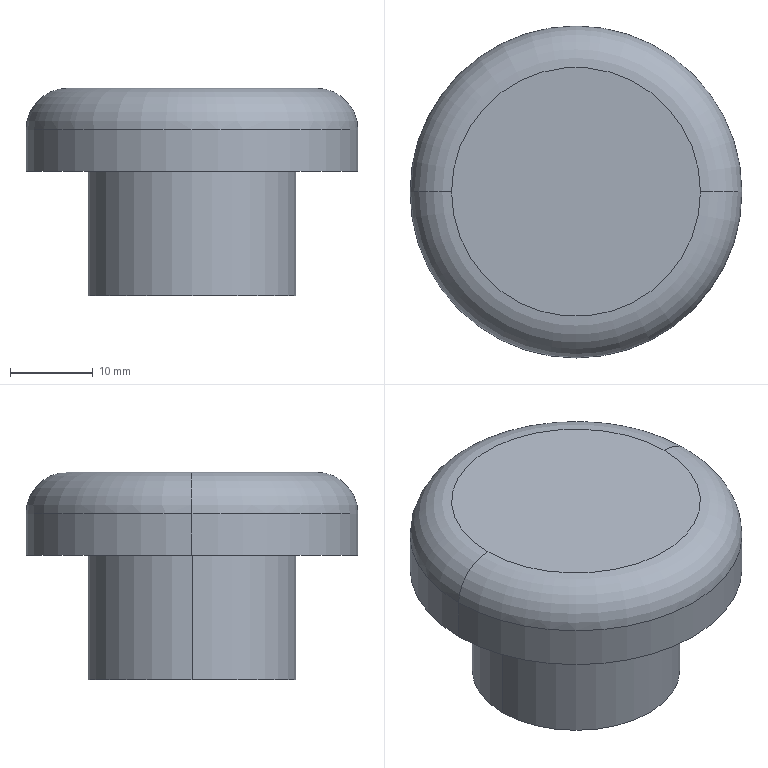Part | STEP file | 7-4-Emergency Stop Button1-619-724_Default | 1 solid | 9 faces | box 40 x 40 x 25 mm | volume 19293 mm3 | cylinder 4 | plane 3 | torus 2 | commonest cylinder face diameters 25 x2 40 x2
STEP:
#1=CARTESIAN_POINT('',(0.,0.,0.));
#2=DIRECTION('',(0.,0.,1.));
#3=DIRECTION('',(1.,0.,0.));
#4=AXIS2_PLACEMENT_3D('',#1,#2,#3);
#5=CARTESIAN_POINT('',(-20.,0.,-5.));
#6=VERTEX_POINT('',#5);
#7=CARTESIAN_POINT('',(20.,0.,-5.));
#8=VERTEX_POINT('',#7);
#9=CARTESIAN_POINT('',(0.,0.,-5.));
#10=DIRECTION('',(0.,0.,-1.));
#11=DIRECTION('',(1.,0.,0.));
#12=AXIS2_PLACEMENT_3D('',#9,#10,#11);
#13=CIRCLE('',#12,20.);
#14=CARTESIAN_POINT('',(0.,0.,-5.));
#15=DIRECTION('',(0.,0.,1.));
#16=DIRECTION('',(1.,0.,0.));
#17=AXIS2_PLACEMENT_3D('',#14,#15,#16);
#18=TOROIDAL_SURFACE('',#17,15.,5.);
#19=CARTESIAN_POINT('',(6.283,0.));
#20=DIRECTION('',(-1.,0.));
#21=VECTOR('',#20,1.);
#22=LINE('',#19,#21);
#23=(GEOMETRIC_REPRESENTATION_CONTEXT(2)PARAMETRIC_REPRESENTATION_CONTEXT()REPRESENTATION_CONTEXT('',''));
#24=DEFINITIONAL_REPRESENTATION('',(#22),#23);
#25=PCURVE('',#18,#24);
#26=CARTESIAN_POINT('',(0.,0.,-25.));
#27=DIRECTION('',(0.,0.,1.));
#28=DIRECTION('',(1.,0.,0.));
#29=AXIS2_PLACEMENT_3D('',#26,#27,#28);
#30=CYLINDRICAL_SURFACE('',#29,20.);
#31=CARTESIAN_POINT('',(6.283,20.));
#32=DIRECTION('',(-1.,0.));
#33=VECTOR('',#32,1.);
#34=LINE('',#31,#33);
#35=(GEOMETRIC_REPRESENTATION_CONTEXT(2)PARAMETRIC_REPRESENTATION_CONTEXT()REPRESENTATION_CONTEXT('',''));
#36=DEFINITIONAL_REPRESENTATION('',(#34),#35);
#37=PCURVE('',#30,#36);
#38=SURFACE_CURVE('',#13,(#25,#37),.PCURVE_S1.);
#39=EDGE_CURVE('',#6,#8,#38,.T.);
#40=ORIENTED_EDGE('',*,*,#39,.F.);
#41=CARTESIAN_POINT('',(-15.,0.,0.));
#42=VERTEX_POINT('',#41);
#43=CARTESIAN_POINT('',(-15.,0.,-5.));
#44=DIRECTION('',(0.,1.,0.));
#45=DIRECTION('',(-1.,0.,0.));
#46=AXIS2_PLACEMENT_3D('',#43,#44,#45);
#47=CIRCLE('',#46,5.);
#48=CARTESIAN_POINT('',(3.142,0.));
#49=DIRECTION('',(0.,1.));
#50=VECTOR('',#49,1.);
#51=LINE('',#48,#50);
#52=(GEOMETRIC_REPRESENTATION_CONTEXT(2)PARAMETRIC_REPRESENTATION_CONTEXT()REPRESENTATION_CONTEXT('',''));
#53=DEFINITIONAL_REPRESENTATION('',(#51),#52);
#54=PCURVE('',#18,#53);
#55=CARTESIAN_POINT('',(0.,0.,-5.));
#56=DIRECTION('',(0.,0.,1.));
#57=DIRECTION('',(1.,0.,0.));
#58=AXIS2_PLACEMENT_3D('',#55,#56,#57);
#59=TOROIDAL_SURFACE('',#58,15.,5.);
#60=CARTESIAN_POINT('',(3.142,0.));
#61=DIRECTION('',(0.,1.));
#62=VECTOR('',#61,1.);
#63=LINE('',#60,#62);
#64=(GEOMETRIC_REPRESENTATION_CONTEXT(2)PARAMETRIC_REPRESENTATION_CONTEXT()REPRESENTATION_CONTEXT('',''));
#65=DEFINITIONAL_REPRESENTATION('',(#63),#64);
#66=PCURVE('',#59,#65);
#67=SURFACE_CURVE('',#47,(#54,#66),.PCURVE_S1.);
#68=EDGE_CURVE('',#6,#42,#67,.T.);
#69=ORIENTED_EDGE('',*,*,#68,.T.);
#70=CARTESIAN_POINT('',(15.,0.,0.));
#71=VERTEX_POINT('',#70);
#72=CARTESIAN_POINT('',(0.,0.,0.));
#73=DIRECTION('',(0.,0.,1.));
#74=DIRECTION('',(1.,0.,0.));
#75=AXIS2_PLACEMENT_3D('',#72,#73,#74);
#76=CIRCLE('',#75,15.);
#77=CARTESIAN_POINT('',(0.,1.571));
#78=DIRECTION('',(1.,0.));
#79=VECTOR('',#78,1.);
#80=LINE('',#77,#79);
#81=(GEOMETRIC_REPRESENTATION_CONTEXT(2)PARAMETRIC_REPRESENTATION_CONTEXT()REPRESENTATION_CONTEXT('',''));
#82=DEFINITIONAL_REPRESENTATION('',(#80),#81);
#83=PCURVE('',#18,#82);
#84=CARTESIAN_POINT('',(0.,0.,0.));
#85=DIRECTION('',(0.,0.,1.));
#86=DIRECTION('',(1.,0.,0.));
#87=AXIS2_PLACEMENT_3D('',#84,#85,#86);
#88=PLANE('',#87);
#89=CARTESIAN_POINT('',(0.,0.));
#90=DIRECTION('',(1.,0.));
#91=AXIS2_PLACEMENT_2D('',#89,#90);
#92=CIRCLE('',#91,15.);
#93=(GEOMETRIC_REPRESENTATION_CONTEXT(2)PARAMETRIC_REPRESENTATION_CONTEXT()REPRESENTATION_CONTEXT('',''));
#94=DEFINITIONAL_REPRESENTATION('',(#92),#93);
#95=PCURVE('',#88,#94);
#96=SURFACE_CURVE('',#76,(#83,#95),.PCURVE_S1.);
#97=EDGE_CURVE('',#71,#42,#96,.T.);
#98=ORIENTED_EDGE('',*,*,#97,.F.);
#99=CARTESIAN_POINT('',(15.,0.,-5.));
#100=DIRECTION('',(0.,-1.,0.));
#101=DIRECTION('',(0.,0.,-1.));
#102=AXIS2_PLACEMENT_3D('',#99,#100,#101);
#103=CIRCLE('',#102,5.);
#104=CARTESIAN_POINT('',(0.,-1.571));
#105=DIRECTION('',(0.,1.));
#106=VECTOR('',#105,1.);
#107=LINE('',#104,#106);
#108=(GEOMETRIC_REPRESENTATION_CONTEXT(2)PARAMETRIC_REPRESENTATION_CONTEXT()REPRESENTATION_CONTEXT('',''));
#109=DEFINITIONAL_REPRESENTATION('',(#107),#108);
#110=PCURVE('',#18,#109);
#111=CARTESIAN_POINT('',(6.283,-1.571));
#112=DIRECTION('',(0.,1.));
#113=VECTOR('',#112,1.);
#114=LINE('',#111,#113);
#115=(GEOMETRIC_REPRESENTATION_CONTEXT(2)PARAMETRIC_REPRESENTATION_CONTEXT()REPRESENTATION_CONTEXT('',''));
#116=DEFINITIONAL_REPRESENTATION('',(#114),#115);
#117=PCURVE('',#59,#116);
#118=SURFACE_CURVE('',#103,(#110,#117),.PCURVE_S1.);
#119=EDGE_CURVE('',#8,#71,#118,.T.);
#120=ORIENTED_EDGE('',*,*,#119,.F.);
#121=EDGE_LOOP('',(#40,#69,#98,#120));
#122=FACE_BOUND('',#121,.T.);
#123=ADVANCED_FACE('',(#122),#18,.T.);
#124=CARTESIAN_POINT('',(-12.5,0.,-10.));
#125=VERTEX_POINT('',#124);
#126=CARTESIAN_POINT('',(12.5,0.,-10.));
#127=VERTEX_POINT('',#126);
#128=CARTESIAN_POINT('',(0.,0.,-10.));
#129=DIRECTION('',(0.,0.,-1.));
#130=DIRECTION('',(-1.,0.,0.));
#131=AXIS2_PLACEMENT_3D('',#128,#129,#130);
#132=CIRCLE('',#131,12.5);
#133=CARTESIAN_POINT('',(0.,0.,-10.));
#134=DIRECTION('',(0.,0.,-1.));
#135=DIRECTION('',(-1.,0.,0.));
#136=AXIS2_PLACEMENT_3D('',#133,#134,#135);
#137=CYLINDRICAL_SURFACE('',#136,12.5);
#138=CARTESIAN_POINT('',(0.,0.));
#139=DIRECTION('',(1.,0.));
#140=VECTOR('',#139,1.);
#141=LINE('',#138,#140);
#142=(GEOMETRIC_REPRESENTATION_CONTEXT(2)PARAMETRIC_REPRESENTATION_CONTEXT()REPRESENTATION_CONTEXT('',''));
#143=DEFINITIONAL_REPRESENTATION('',(#141),#142);
#144=PCURVE('',#137,#143);
#145=CARTESIAN_POINT('',(0.,0.,-10.));
#146=DIRECTION('',(0.,0.,-1.));
#147=DIRECTION('',(-1.,0.,0.));
#148=AXIS2_PLACEMENT_3D('',#145,#146,#147);
#149=PLANE('',#148);
#150=CARTESIAN_POINT('',(0.,0.));
#151=DIRECTION('',(1.,0.));
#152=AXIS2_PLACEMENT_2D('',#150,#151);
#153=CIRCLE('',#152,12.5);
#154=(GEOMETRIC_REPRESENTATION_CONTEXT(2)PARAMETRIC_REPRESENTATION_CONTEXT()REPRESENTATION_CONTEXT('',''));
#155=DEFINITIONAL_REPRESENTATION('',(#153),#154);
#156=PCURVE('',#149,#155);
#157=SURFACE_CURVE('',#132,(#144,#156),.PCURVE_S1.);
#158=EDGE_CURVE('',#125,#127,#157,.T.);
#159=ORIENTED_EDGE('',*,*,#158,.T.);
#160=CARTESIAN_POINT('',(12.5,0.,-25.));
#161=VERTEX_POINT('',#160);
#162=CARTESIAN_POINT('',(12.5,0.,-10.));
#163=DIRECTION('',(0.,0.,-1.));
#164=VECTOR('',#163,1.);
#165=LINE('',#162,#164);
#166=CARTESIAN_POINT('',(3.142,0.));
#167=DIRECTION('',(0.,1.));
#168=VECTOR('',#167,1.);
#169=LINE('',#166,#168);
#170=(GEOMETRIC_REPRESENTATION_CONTEXT(2)PARAMETRIC_REPRESENTATION_CONTEXT()REPRESENTATION_CONTEXT('',''));
#171=DEFINITIONAL_REPRESENTATION('',(#169),#170);
#172=PCURVE('',#137,#171);
#173=CARTESIAN_POINT('',(0.,0.,-10.));
#174=DIRECTION('',(0.,0.,-1.));
#175=DIRECTION('',(-1.,0.,0.));
#176=AXIS2_PLACEMENT_3D('',#173,#174,#175);
#177=CYLINDRICAL_SURFACE('',#176,12.5);
#178=CARTESIAN_POINT('',(3.142,0.));
#179=DIRECTION('',(0.,1.));
#180=VECTOR('',#179,1.);
#181=LINE('',#178,#180);
#182=(GEOMETRIC_REPRESENTATION_CONTEXT(2)PARAMETRIC_REPRESENTATION_CONTEXT()REPRESENTATION_CONTEXT('',''));
#183=DEFINITIONAL_REPRESENTATION('',(#181),#182);
#184=PCURVE('',#177,#183);
#185=SURFACE_CURVE('',#165,(#172,#184),.PCURVE_S1.);
#186=EDGE_CURVE('',#127,#161,#185,.T.);
#187=ORIENTED_EDGE('',*,*,#186,.T.);
#188=CARTESIAN_POINT('',(-12.5,0.,-25.));
#189=VERTEX_POINT('',#188);
#190=CARTESIAN_POINT('',(0.,0.,-25.));
#191=DIRECTION('',(0.,0.,-1.));
#192=DIRECTION('',(-1.,0.,0.));
#193=AXIS2_PLACEMENT_3D('',#190,#191,#192);
#194=CIRCLE('',#193,12.5);
#195=CARTESIAN_POINT('',(0.,15.));
#196=DIRECTION('',(1.,0.));
#197=VECTOR('',#196,1.);
#198=LINE('',#195,#197);
#199=(GEOMETRIC_REPRESENTATION_CONTEXT(2)PARAMETRIC_REPRESENTATION_CONTEXT()REPRESENTATION_CONTEXT('',''));
#200=DEFINITIONAL_REPRESENTATION('',(#198),#199);
#201=PCURVE('',#137,#200);
#202=CARTESIAN_POINT('',(0.,0.,-25.));
#203=DIRECTION('',(0.,0.,1.));
#204=DIRECTION('',(1.,0.,0.));
#205=AXIS2_PLACEMENT_3D('',#202,#203,#204);
#206=PLANE('',#205);
#207=CARTESIAN_POINT('',(-12.5,0.));
#208=CARTESIAN_POINT('',(-12.5,21.651));
#209=CARTESIAN_POINT('',(6.25,10.825));
#210=CARTESIAN_POINT('',(25.,0.));
#211=CARTESIAN_POINT('',(6.25,-10.825));
#212=CARTESIAN_POINT('',(-12.5,-21.651));
#213=CARTESIAN_POINT('',(-12.5,0.));
#214=(BOUNDED_CURVE()B_SPLINE_CURVE(2,(#207,#208,#209,#210,#211,#212,#213),.UNSPECIFIED.,.T.,.F.)B_SPLINE_CURVE_WITH_KNOTS((1,2,2,2,2,1),(-2.094,0.,2.094,4.189,6.283,8.378),.UNSPECIFIED.)CURVE()GEOMETRIC_REPRESENTATION_ITEM()RATIONAL_B_SPLINE_CURVE((1.,0.5,1.,0.5,1.,0.5,1.))REPRESENTATION_ITEM(''));
#215=(GEOMETRIC_REPRESENTATION_CONTEXT(2)PARAMETRIC_REPRESENTATION_CONTEXT()REPRESENTATION_CONTEXT('',''));
#216=DEFINITIONAL_REPRESENTATION('',(#214),#215);
#217=PCURVE('',#206,#216);
#218=SURFACE_CURVE('',#194,(#201,#217),.PCURVE_S1.);
#219=EDGE_CURVE('',#189,#161,#218,.T.);
#220=ORIENTED_EDGE('',*,*,#219,.F.);
#221=CARTESIAN_POINT('',(-12.5,0.,-10.));
#222=DIRECTION('',(0.,0.,-1.));
#223=VECTOR('',#222,1.);
#224=LINE('',#221,#223);
#225=CARTESIAN_POINT('',(0.,0.));
#226=DIRECTION('',(0.,1.));
#227=VECTOR('',#226,1.);
#228=LINE('',#225,#227);
#229=(GEOMETRIC_REPRESENTATION_CONTEXT(2)PARAMETRIC_REPRESENTATION_CONTEXT()REPRESENTATION_CONTEXT('',''));
#230=DEFINITIONAL_REPRESENTATION('',(#228),#229);
#231=PCURVE('',#137,#230);
#232=CARTESIAN_POINT('',(6.283,0.));
#233=DIRECTION('',(0.,1.));
#234=VECTOR('',#233,1.);
#235=LINE('',#232,#234);
#236=(GEOMETRIC_REPRESENTATION_CONTEXT(2)PARAMETRIC_REPRESENTATION_CONTEXT()REPRESENTATION_CONTEXT('',''));
#237=DEFINITIONAL_REPRESENTATION('',(#235),#236);
#238=PCURVE('',#177,#237);
#239=SURFACE_CURVE('',#224,(#231,#238),.PCURVE_S1.);
#240=EDGE_CURVE('',#125,#189,#239,.T.);
#241=ORIENTED_EDGE('',*,*,#240,.F.);
#242=EDGE_LOOP('',(#159,#187,#220,#241));
#243=FACE_BOUND('',#242,.T.);
#244=ADVANCED_FACE('',(#243),#137,.T.);
#245=CARTESIAN_POINT('',(20.,0.,-10.));
#246=VERTEX_POINT('',#245);
#247=CARTESIAN_POINT('',(-20.,0.,-10.));
#248=VERTEX_POINT('',#247);
#249=CARTESIAN_POINT('',(0.,0.,-10.));
#250=DIRECTION('',(0.,0.,1.));
#251=DIRECTION('',(-1.,0.,0.));
#252=AXIS2_PLACEMENT_3D('',#249,#250,#251);
#253=CIRCLE('',#252,20.);
#254=CARTESIAN_POINT('',(-3.142,15.));
#255=DIRECTION('',(1.,0.));
#256=VECTOR('',#255,1.);
#257=LINE('',#254,#256);
#258=(GEOMETRIC_REPRESENTATION_CONTEXT(2)PARAMETRIC_REPRESENTATION_CONTEXT()REPRESENTATION_CONTEXT('',''));
#259=DEFINITIONAL_REPRESENTATION('',(#257),#258);
#260=PCURVE('',#30,#259);
#261=CARTESIAN_POINT('',(20.,0.));
#262=CARTESIAN_POINT('',(20.,-34.641));
#263=CARTESIAN_POINT('',(-10.,-17.321));
#264=CARTESIAN_POINT('',(-40.,0.));
#265=CARTESIAN_POINT('',(-10.,17.321));
#266=CARTESIAN_POINT('',(20.,34.641));
#267=CARTESIAN_POINT('',(20.,0.));
#268=(BOUNDED_CURVE()B_SPLINE_CURVE(2,(#261,#262,#263,#264,#265,#266,#267),.UNSPECIFIED.,.T.,.F.)B_SPLINE_CURVE_WITH_KNOTS((1,2,2,2,2,1),(-2.094,0.,2.094,4.189,6.283,8.378),.UNSPECIFIED.)CURVE()GEOMETRIC_REPRESENTATION_ITEM()RATIONAL_B_SPLINE_CURVE((1.,0.5,1.,0.5,1.,0.5,1.))REPRESENTATION_ITEM(''));
#269=(GEOMETRIC_REPRESENTATION_CONTEXT(2)PARAMETRIC_REPRESENTATION_CONTEXT()REPRESENTATION_CONTEXT('',''));
#270=DEFINITIONAL_REPRESENTATION('',(#268),#269);
#271=PCURVE('',#149,#270);
#272=SURFACE_CURVE('',#253,(#260,#271),.PCURVE_S1.);
#273=EDGE_CURVE('',#246,#248,#272,.T.);
#274=ORIENTED_EDGE('',*,*,#273,.T.);
#275=CARTESIAN_POINT('',(-20.,0.,-25.));
#276=DIRECTION('',(0.,0.,1.));
#277=VECTOR('',#276,1.);
#278=LINE('',#275,#277);
#279=CARTESIAN_POINT('',(3.142,0.));
#280=DIRECTION('',(0.,1.));
#281=VECTOR('',#280,1.);
#282=LINE('',#279,#281);
#283=(GEOMETRIC_REPRESENTATION_CONTEXT(2)PARAMETRIC_REPRESENTATION_CONTEXT()REPRESENTATION_CONTEXT('',''));
#284=DEFINITIONAL_REPRESENTATION('',(#282),#283);
#285=PCURVE('',#30,#284);
#286=CARTESIAN_POINT('',(0.,0.,-25.));
#287=DIRECTION('',(0.,0.,1.));
#288=DIRECTION('',(1.,0.,0.));
#289=AXIS2_PLACEMENT_3D('',#286,#287,#288);
#290=CYLINDRICAL_SURFACE('',#289,20.);
#291=CARTESIAN_POINT('',(3.142,0.));
#292=DIRECTION('',(0.,1.));
#293=VECTOR('',#292,1.);
#294=LINE('',#291,#293);
#295=(GEOMETRIC_REPRESENTATION_CONTEXT(2)PARAMETRIC_REPRESENTATION_CONTEXT()REPRESENTATION_CONTEXT('',''));
#296=DEFINITIONAL_REPRESENTATION('',(#294),#295);
#297=PCURVE('',#290,#296);
#298=SURFACE_CURVE('',#278,(#285,#297),.PCURVE_S1.);
#299=EDGE_CURVE('',#248,#6,#298,.T.);
#300=ORIENTED_EDGE('',*,*,#299,.T.);
#301=ORIENTED_EDGE('',*,*,#39,.T.);
#302=CARTESIAN_POINT('',(20.,0.,-25.));
#303=DIRECTION('',(0.,0.,1.));
#304=VECTOR('',#303,1.);
#305=LINE('',#302,#304);
#306=CARTESIAN_POINT('',(0.,0.));
#307=DIRECTION('',(0.,1.));
#308=VECTOR('',#307,1.);
#309=LINE('',#306,#308);
#310=(GEOMETRIC_REPRESENTATION_CONTEXT(2)PARAMETRIC_REPRESENTATION_CONTEXT()REPRESENTATION_CONTEXT('',''));
#311=DEFINITIONAL_REPRESENTATION('',(#309),#310);
#312=PCURVE('',#30,#311);
#313=CARTESIAN_POINT('',(6.283,0.));
#314=DIRECTION('',(0.,1.));
#315=VECTOR('',#314,1.);
#316=LINE('',#313,#315);
#317=(GEOMETRIC_REPRESENTATION_CONTEXT(2)PARAMETRIC_REPRESENTATION_CONTEXT()REPRESENTATION_CONTEXT('',''));
#318=DEFINITIONAL_REPRESENTATION('',(#316),#317);
#319=PCURVE('',#290,#318);
#320=SURFACE_CURVE('',#305,(#312,#319),.PCURVE_S1.);
#321=EDGE_CURVE('',#246,#8,#320,.T.);
#322=ORIENTED_EDGE('',*,*,#321,.F.);
#323=EDGE_LOOP('',(#274,#300,#301,#322));
#324=FACE_BOUND('',#323,.T.);
#325=ADVANCED_FACE('',(#324),#30,.T.);
#326=ORIENTED_EDGE('',*,*,#299,.F.);
#327=CARTESIAN_POINT('',(0.,0.,-10.));
#328=DIRECTION('',(0.,0.,1.));
#329=DIRECTION('',(-1.,0.,0.));
#330=AXIS2_PLACEMENT_3D('',#327,#328,#329);
#331=CIRCLE('',#330,20.);
#332=CARTESIAN_POINT('',(3.142,15.));
#333=DIRECTION('',(1.,0.));
#334=VECTOR('',#333,1.);
#335=LINE('',#332,#334);
#336=(GEOMETRIC_REPRESENTATION_CONTEXT(2)PARAMETRIC_REPRESENTATION_CONTEXT()REPRESENTATION_CONTEXT('',''));
#337=DEFINITIONAL_REPRESENTATION('',(#335),#336);
#338=PCURVE('',#290,#337);
#339=CARTESIAN_POINT('',(20.,0.));
#340=CARTESIAN_POINT('',(20.,-34.641));
#341=CARTESIAN_POINT('',(-10.,-17.321));
#342=CARTESIAN_POINT('',(-40.,0.));
#343=CARTESIAN_POINT('',(-10.,17.321));
#344=CARTESIAN_POINT('',(20.,34.641));
#345=CARTESIAN_POINT('',(20.,0.));
#346=(BOUNDED_CURVE()B_SPLINE_CURVE(2,(#339,#340,#341,#342,#343,#344,#345),.UNSPECIFIED.,.T.,.F.)B_SPLINE_CURVE_WITH_KNOTS((1,2,2,2,2,1),(-2.094,0.,2.094,4.189,6.283,8.378),.UNSPECIFIED.)CURVE()GEOMETRIC_REPRESENTATION_ITEM()RATIONAL_B_SPLINE_CURVE((1.,0.5,1.,0.5,1.,0.5,1.))REPRESENTATION_ITEM(''));
#347=(GEOMETRIC_REPRESENTATION_CONTEXT(2)PARAMETRIC_REPRESENTATION_CONTEXT()REPRESENTATION_CONTEXT('',''));
#348=DEFINITIONAL_REPRESENTATION('',(#346),#347);
#349=PCURVE('',#149,#348);
#350=SURFACE_CURVE('',#331,(#338,#349),.PCURVE_S1.);
#351=EDGE_CURVE('',#248,#246,#350,.T.);
#352=ORIENTED_EDGE('',*,*,#351,.T.);
#353=ORIENTED_EDGE('',*,*,#321,.T.);
#354=CARTESIAN_POINT('',(0.,0.,-5.));
#355=DIRECTION('',(0.,0.,-1.));
#356=DIRECTION('',(1.,0.,0.));
#357=AXIS2_PLACEMENT_3D('',#354,#355,#356);
#358=CIRCLE('',#357,20.);
#359=CARTESIAN_POINT('',(6.283,20.));
#360=DIRECTION('',(-1.,0.));
#361=VECTOR('',#360,1.);
#362=LINE('',#359,#361);
#363=(GEOMETRIC_REPRESENTATION_CONTEXT(2)PARAMETRIC_REPRESENTATION_CONTEXT()REPRESENTATION_CONTEXT('',''));
#364=DEFINITIONAL_REPRESENTATION('',(#362),#363);
#365=PCURVE('',#290,#364);
#366=CARTESIAN_POINT('',(6.283,0.));
#367=DIRECTION('',(-1.,0.));
#368=VECTOR('',#367,1.);
#369=LINE('',#366,#368);
#370=(GEOMETRIC_REPRESENTATION_CONTEXT(2)PARAMETRIC_REPRESENTATION_CONTEXT()REPRESENTATION_CONTEXT('',''));
#371=DEFINITIONAL_REPRESENTATION('',(#369),#370);
#372=PCURVE('',#59,#371);
#373=SURFACE_CURVE('',#358,(#365,#372),.PCURVE_S1.);
#374=EDGE_CURVE('',#8,#6,#373,.T.);
#375=ORIENTED_EDGE('',*,*,#374,.T.);
#376=EDGE_LOOP('',(#326,#352,#353,#375));
#377=FACE_BOUND('',#376,.T.);
#378=ADVANCED_FACE('',(#377),#290,.T.);
#379=ORIENTED_EDGE('',*,*,#97,.T.);
#380=CARTESIAN_POINT('',(0.,0.,0.));
#381=DIRECTION('',(0.,0.,1.));
#382=DIRECTION('',(1.,0.,0.));
#383=AXIS2_PLACEMENT_3D('',#380,#381,#382);
#384=CIRCLE('',#383,15.);
#385=CARTESIAN_POINT('',(0.,0.));
#386=DIRECTION('',(1.,0.));
#387=AXIS2_PLACEMENT_2D('',#385,#386);
#388=CIRCLE('',#387,15.);
#389=(GEOMETRIC_REPRESENTATION_CONTEXT(2)PARAMETRIC_REPRESENTATION_CONTEXT()REPRESENTATION_CONTEXT('',''));
#390=DEFINITIONAL_REPRESENTATION('',(#388),#389);
#391=PCURVE('',#88,#390);
#392=CARTESIAN_POINT('',(0.,1.571));
#393=DIRECTION('',(1.,0.));
#394=VECTOR('',#393,1.);
#395=LINE('',#392,#394);
#396=(GEOMETRIC_REPRESENTATION_CONTEXT(2)PARAMETRIC_REPRESENTATION_CONTEXT()REPRESENTATION_CONTEXT('',''));
#397=DEFINITIONAL_REPRESENTATION('',(#395),#396);
#398=PCURVE('',#59,#397);
#399=SURFACE_CURVE('',#384,(#391,#398),.PCURVE_S1.);
#400=EDGE_CURVE('',#42,#71,#399,.T.);
#401=ORIENTED_EDGE('',*,*,#400,.T.);
#402=EDGE_LOOP('',(#379,#401));
#403=FACE_BOUND('',#402,.T.);
#404=ADVANCED_FACE('',(#403),#88,.T.);
#405=ORIENTED_EDGE('',*,*,#273,.F.);
#406=ORIENTED_EDGE('',*,*,#351,.F.);
#407=EDGE_LOOP('',(#405,#406));
#408=FACE_BOUND('',#407,.T.);
#409=ORIENTED_EDGE('',*,*,#158,.F.);
#410=CARTESIAN_POINT('',(0.,0.,-10.));
#411=DIRECTION('',(0.,0.,-1.));
#412=DIRECTION('',(-1.,0.,0.));
#413=AXIS2_PLACEMENT_3D('',#410,#411,#412);
#414=CIRCLE('',#413,12.5);
#415=CARTESIAN_POINT('',(0.,0.));
#416=DIRECTION('',(1.,0.));
#417=AXIS2_PLACEMENT_2D('',#415,#416);
#418=CIRCLE('',#417,12.5);
#419=(GEOMETRIC_REPRESENTATION_CONTEXT(2)PARAMETRIC_REPRESENTATION_CONTEXT()REPRESENTATION_CONTEXT('',''));
#420=DEFINITIONAL_REPRESENTATION('',(#418),#419);
#421=PCURVE('',#149,#420);
#422=CARTESIAN_POINT('',(0.,0.));
#423=DIRECTION('',(1.,0.));
#424=VECTOR('',#423,1.);
#425=LINE('',#422,#424);
#426=(GEOMETRIC_REPRESENTATION_CONTEXT(2)PARAMETRIC_REPRESENTATION_CONTEXT()REPRESENTATION_CONTEXT('',''));
#427=DEFINITIONAL_REPRESENTATION('',(#425),#426);
#428=PCURVE('',#177,#427);
#429=SURFACE_CURVE('',#414,(#421,#428),.PCURVE_S1.);
#430=EDGE_CURVE('',#127,#125,#429,.T.);
#431=ORIENTED_EDGE('',*,*,#430,.F.);
#432=EDGE_LOOP('',(#409,#431));
#433=FACE_BOUND('',#432,.T.);
#434=ADVANCED_FACE('',(#408,#433),#149,.T.);
#435=ORIENTED_EDGE('',*,*,#186,.F.);
#436=ORIENTED_EDGE('',*,*,#430,.T.);
#437=ORIENTED_EDGE('',*,*,#240,.T.);
#438=CARTESIAN_POINT('',(0.,0.,-25.));
#439=DIRECTION('',(0.,0.,-1.));
#440=DIRECTION('',(-1.,0.,0.));
#441=AXIS2_PLACEMENT_3D('',#438,#439,#440);
#442=CIRCLE('',#441,12.5);
#443=CARTESIAN_POINT('',(0.,15.));
#444=DIRECTION('',(1.,0.));
#445=VECTOR('',#444,1.);
#446=LINE('',#443,#445);
#447=(GEOMETRIC_REPRESENTATION_CONTEXT(2)PARAMETRIC_REPRESENTATION_CONTEXT()REPRESENTATION_CONTEXT('',''));
#448=DEFINITIONAL_REPRESENTATION('',(#446),#447);
#449=PCURVE('',#177,#448);
#450=CARTESIAN_POINT('',(-12.5,0.));
#451=CARTESIAN_POINT('',(-12.5,21.651));
#452=CARTESIAN_POINT('',(6.25,10.825));
#453=CARTESIAN_POINT('',(25.,0.));
#454=CARTESIAN_POINT('',(6.25,-10.825));
#455=CARTESIAN_POINT('',(-12.5,-21.651));
#456=CARTESIAN_POINT('',(-12.5,0.));
#457=(BOUNDED_CURVE()B_SPLINE_CURVE(2,(#450,#451,#452,#453,#454,#455,#456),.UNSPECIFIED.,.T.,.F.)B_SPLINE_CURVE_WITH_KNOTS((1,2,2,2,2,1),(-2.094,0.,2.094,4.189,6.283,8.378),.UNSPECIFIED.)CURVE()GEOMETRIC_REPRESENTATION_ITEM()RATIONAL_B_SPLINE_CURVE((1.,0.5,1.,0.5,1.,0.5,1.))REPRESENTATION_ITEM(''));
#458=(GEOMETRIC_REPRESENTATION_CONTEXT(2)PARAMETRIC_REPRESENTATION_CONTEXT()REPRESENTATION_CONTEXT('',''));
#459=DEFINITIONAL_REPRESENTATION('',(#457),#458);
#460=PCURVE('',#206,#459);
#461=SURFACE_CURVE('',#442,(#449,#460),.PCURVE_S1.);
#462=EDGE_CURVE('',#161,#189,#461,.T.);
#463=ORIENTED_EDGE('',*,*,#462,.F.);
#464=EDGE_LOOP('',(#435,#436,#437,#463));
#465=FACE_BOUND('',#464,.T.);
#466=ADVANCED_FACE('',(#465),#177,.T.);
#467=ORIENTED_EDGE('',*,*,#219,.T.);
#468=ORIENTED_EDGE('',*,*,#462,.T.);
#469=EDGE_LOOP('',(#467,#468));
#470=FACE_BOUND('',#469,.T.);
#471=ADVANCED_FACE('',(#470),#206,.F.);
#472=ORIENTED_EDGE('',*,*,#68,.F.);
#473=ORIENTED_EDGE('',*,*,#374,.F.);
#474=ORIENTED_EDGE('',*,*,#119,.T.);
#475=ORIENTED_EDGE('',*,*,#400,.F.);
#476=EDGE_LOOP('',(#472,#473,#474,#475));
#477=FACE_BOUND('',#476,.T.);
#478=ADVANCED_FACE('',(#477),#59,.T.);
#479=CLOSED_SHELL('',(#123,#244,#325,#378,#404,#434,#466,#471,#478));
#480=MANIFOLD_SOLID_BREP('',#479);
#481=(LENGTH_UNIT()NAMED_UNIT(*)SI_UNIT(.MILLI.,.METRE.));
#482=UNCERTAINTY_MEASURE_WITH_UNIT(LENGTH_MEASURE(0.0000001),#481,'','');
#483=(NAMED_UNIT(*)PLANE_ANGLE_UNIT()SI_UNIT($,.RADIAN.));
#484=(NAMED_UNIT(*)SI_UNIT($,.STERADIAN.)SOLID_ANGLE_UNIT());
#485=(GEOMETRIC_REPRESENTATION_CONTEXT(3)GLOBAL_UNCERTAINTY_ASSIGNED_CONTEXT((#482))GLOBAL_UNIT_ASSIGNED_CONTEXT((#481,#483,#484))REPRESENTATION_CONTEXT('',''));
#486=ADVANCED_BREP_SHAPE_REPRESENTATION('',(#4,#480),#485);